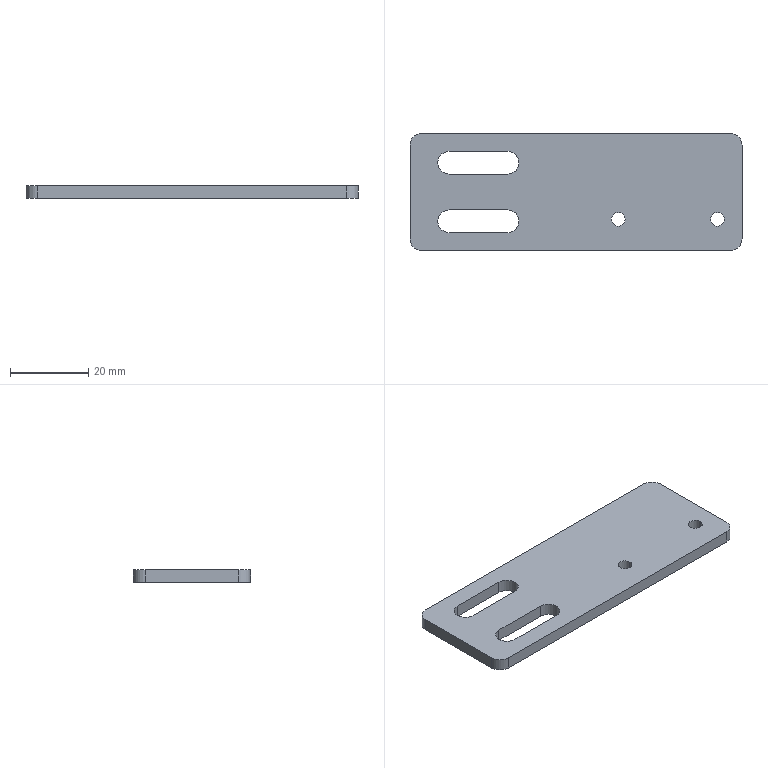Part | STEP file | J014-EBZ05-17-06 | 1 solid | 24 faces | box 85 x 30 x 3.2 mm | volume 7348 mm3 | cylinder 14 | plane 10 | commonest cylinder face diameters 5.8 x6 3.5 x4 6 x4
STEP:
#1=CARTESIAN_POINT('',(76.95,8.,0.));
#2=VERTEX_POINT('',#1);
#3=CARTESIAN_POINT('',(80.45,8.,0.));
#4=VERTEX_POINT('',#3);
#5=CARTESIAN_POINT('',(78.7,8.,0.));
#6=DIRECTION('',(0.,0.,1.));
#7=DIRECTION('',(1.,0.,0.));
#8=AXIS2_PLACEMENT_3D('',#5,#6,#7);
#9=CIRCLE('',#8,1.75);
#10=EDGE_CURVE('',#2,#4,#9,.T.);
#11=ORIENTED_EDGE('',*,*,#10,.F.);
#12=CARTESIAN_POINT('',(76.95,8.,3.2));
#13=VERTEX_POINT('',#12);
#14=CARTESIAN_POINT('',(76.95,8.,0.));
#15=DIRECTION('',(0.,0.,1.));
#16=VECTOR('',#15,1000.);
#17=LINE('',#14,#16);
#18=EDGE_CURVE('',#2,#13,#17,.T.);
#19=ORIENTED_EDGE('',*,*,#18,.T.);
#20=CARTESIAN_POINT('',(80.45,8.,3.2));
#21=VERTEX_POINT('',#20);
#22=CARTESIAN_POINT('',(78.7,8.,3.2));
#23=DIRECTION('',(0.,0.,-1.));
#24=DIRECTION('',(-1.,0.,0.));
#25=AXIS2_PLACEMENT_3D('',#22,#23,#24);
#26=CIRCLE('',#25,1.75);
#27=EDGE_CURVE('',#21,#13,#26,.T.);
#28=ORIENTED_EDGE('',*,*,#27,.F.);
#29=CARTESIAN_POINT('',(80.45,8.,0.));
#30=DIRECTION('',(0.,0.,1.));
#31=VECTOR('',#30,1000.);
#32=LINE('',#29,#31);
#33=EDGE_CURVE('',#4,#21,#32,.T.);
#34=ORIENTED_EDGE('',*,*,#33,.F.);
#35=EDGE_LOOP('',(#11,#19,#28,#34));
#36=FACE_OUTER_BOUND('',#35,.T.);
#37=CARTESIAN_POINT('',(78.7,8.,0.));
#38=DIRECTION('',(0.,0.,1.));
#39=DIRECTION('',(1.,0.,0.));
#40=AXIS2_PLACEMENT_3D('',#37,#38,#39);
#41=CYLINDRICAL_SURFACE('',#40,1.75);
#42=ADVANCED_FACE('',(#36),#41,.F.);
#43=CARTESIAN_POINT('',(51.55,8.,0.));
#44=VERTEX_POINT('',#43);
#45=CARTESIAN_POINT('',(55.05,8.,0.));
#46=VERTEX_POINT('',#45);
#47=CARTESIAN_POINT('',(53.3,8.,0.));
#48=DIRECTION('',(0.,0.,1.));
#49=DIRECTION('',(1.,0.,0.));
#50=AXIS2_PLACEMENT_3D('',#47,#48,#49);
#51=CIRCLE('',#50,1.75);
#52=EDGE_CURVE('',#44,#46,#51,.T.);
#53=ORIENTED_EDGE('',*,*,#52,.F.);
#54=CARTESIAN_POINT('',(51.55,8.,3.2));
#55=VERTEX_POINT('',#54);
#56=CARTESIAN_POINT('',(51.55,8.,0.));
#57=DIRECTION('',(0.,0.,1.));
#58=VECTOR('',#57,1000.);
#59=LINE('',#56,#58);
#60=EDGE_CURVE('',#44,#55,#59,.T.);
#61=ORIENTED_EDGE('',*,*,#60,.T.);
#62=CARTESIAN_POINT('',(55.05,8.,3.2));
#63=VERTEX_POINT('',#62);
#64=CARTESIAN_POINT('',(53.3,8.,3.2));
#65=DIRECTION('',(0.,0.,-1.));
#66=DIRECTION('',(-1.,0.,0.));
#67=AXIS2_PLACEMENT_3D('',#64,#65,#66);
#68=CIRCLE('',#67,1.75);
#69=EDGE_CURVE('',#63,#55,#68,.T.);
#70=ORIENTED_EDGE('',*,*,#69,.F.);
#71=CARTESIAN_POINT('',(55.05,8.,0.));
#72=DIRECTION('',(0.,0.,1.));
#73=VECTOR('',#72,1000.);
#74=LINE('',#71,#73);
#75=EDGE_CURVE('',#46,#63,#74,.T.);
#76=ORIENTED_EDGE('',*,*,#75,.F.);
#77=EDGE_LOOP('',(#53,#61,#70,#76));
#78=FACE_OUTER_BOUND('',#77,.T.);
#79=CARTESIAN_POINT('',(53.3,8.,0.));
#80=DIRECTION('',(0.,0.,1.));
#81=DIRECTION('',(1.,0.,0.));
#82=AXIS2_PLACEMENT_3D('',#79,#80,#81);
#83=CYLINDRICAL_SURFACE('',#82,1.75);
#84=ADVANCED_FACE('',(#78),#83,.F.);
#85=CARTESIAN_POINT('',(7.1,22.5,3.2));
#86=VERTEX_POINT('',#85);
#87=CARTESIAN_POINT('',(10.,25.4,3.2));
#88=VERTEX_POINT('',#87);
#89=CARTESIAN_POINT('',(10.,22.5,3.2));
#90=DIRECTION('',(0.,0.,-1.));
#91=DIRECTION('',(-1.,0.,0.));
#92=AXIS2_PLACEMENT_3D('',#89,#90,#91);
#93=CIRCLE('',#92,2.9);
#94=EDGE_CURVE('',#86,#88,#93,.T.);
#95=ORIENTED_EDGE('',*,*,#94,.F.);
#96=CARTESIAN_POINT('',(7.1,22.5,0.));
#97=VERTEX_POINT('',#96);
#98=CARTESIAN_POINT('',(7.1,22.5,3.2));
#99=DIRECTION('',(0.,0.,-1.));
#100=VECTOR('',#99,1000.);
#101=LINE('',#98,#100);
#102=EDGE_CURVE('',#86,#97,#101,.T.);
#103=ORIENTED_EDGE('',*,*,#102,.T.);
#104=CARTESIAN_POINT('',(10.,25.4,0.));
#105=VERTEX_POINT('',#104);
#106=CARTESIAN_POINT('',(10.,22.5,0.));
#107=DIRECTION('',(0.,0.,1.));
#108=DIRECTION('',(1.,0.,0.));
#109=AXIS2_PLACEMENT_3D('',#106,#107,#108);
#110=CIRCLE('',#109,2.9);
#111=EDGE_CURVE('',#105,#97,#110,.T.);
#112=ORIENTED_EDGE('',*,*,#111,.F.);
#113=CARTESIAN_POINT('',(10.,25.4,3.2));
#114=DIRECTION('',(0.,0.,-1.));
#115=VECTOR('',#114,1000.);
#116=LINE('',#113,#115);
#117=EDGE_CURVE('',#88,#105,#116,.T.);
#118=ORIENTED_EDGE('',*,*,#117,.F.);
#119=EDGE_LOOP('',(#95,#103,#112,#118));
#120=FACE_OUTER_BOUND('',#119,.T.);
#121=CARTESIAN_POINT('',(10.,22.5,3.2));
#122=DIRECTION('',(0.,0.,-1.));
#123=DIRECTION('',(-1.,0.,0.));
#124=AXIS2_PLACEMENT_3D('',#121,#122,#123);
#125=CYLINDRICAL_SURFACE('',#124,2.9);
#126=ADVANCED_FACE('',(#120),#125,.F.);
#127=CARTESIAN_POINT('',(7.1,7.5,3.2));
#128=VERTEX_POINT('',#127);
#129=CARTESIAN_POINT('',(10.,10.4,3.2));
#130=VERTEX_POINT('',#129);
#131=CARTESIAN_POINT('',(10.,7.5,3.2));
#132=DIRECTION('',(0.,0.,-1.));
#133=DIRECTION('',(-1.,0.,0.));
#134=AXIS2_PLACEMENT_3D('',#131,#132,#133);
#135=CIRCLE('',#134,2.9);
#136=EDGE_CURVE('',#128,#130,#135,.T.);
#137=ORIENTED_EDGE('',*,*,#136,.F.);
#138=CARTESIAN_POINT('',(7.1,7.5,0.));
#139=VERTEX_POINT('',#138);
#140=CARTESIAN_POINT('',(7.1,7.5,3.2));
#141=DIRECTION('',(0.,0.,-1.));
#142=VECTOR('',#141,1000.);
#143=LINE('',#140,#142);
#144=EDGE_CURVE('',#128,#139,#143,.T.);
#145=ORIENTED_EDGE('',*,*,#144,.T.);
#146=CARTESIAN_POINT('',(10.,10.4,0.));
#147=VERTEX_POINT('',#146);
#148=CARTESIAN_POINT('',(10.,7.5,0.));
#149=DIRECTION('',(0.,0.,1.));
#150=DIRECTION('',(1.,0.,0.));
#151=AXIS2_PLACEMENT_3D('',#148,#149,#150);
#152=CIRCLE('',#151,2.9);
#153=EDGE_CURVE('',#147,#139,#152,.T.);
#154=ORIENTED_EDGE('',*,*,#153,.F.);
#155=CARTESIAN_POINT('',(10.,10.4,3.2));
#156=DIRECTION('',(0.,0.,-1.));
#157=VECTOR('',#156,1000.);
#158=LINE('',#155,#157);
#159=EDGE_CURVE('',#130,#147,#158,.T.);
#160=ORIENTED_EDGE('',*,*,#159,.F.);
#161=EDGE_LOOP('',(#137,#145,#154,#160));
#162=FACE_OUTER_BOUND('',#161,.T.);
#163=CARTESIAN_POINT('',(10.,7.5,3.2));
#164=DIRECTION('',(0.,0.,-1.));
#165=DIRECTION('',(-1.,0.,0.));
#166=AXIS2_PLACEMENT_3D('',#163,#164,#165);
#167=CYLINDRICAL_SURFACE('',#166,2.9);
#168=ADVANCED_FACE('',(#162),#167,.F.);
#169=CARTESIAN_POINT('',(78.7,8.,0.));
#170=DIRECTION('',(0.,0.,1.));
#171=DIRECTION('',(1.,0.,0.));
#172=AXIS2_PLACEMENT_3D('',#169,#170,#171);
#173=CIRCLE('',#172,1.75);
#174=EDGE_CURVE('',#4,#2,#173,.T.);
#175=ORIENTED_EDGE('',*,*,#174,.T.);
#176=ORIENTED_EDGE('',*,*,#10,.T.);
#177=EDGE_LOOP('',(#175,#176));
#178=FACE_BOUND('',#177,.T.);
#179=CARTESIAN_POINT('',(53.3,8.,0.));
#180=DIRECTION('',(0.,0.,1.));
#181=DIRECTION('',(1.,0.,0.));
#182=AXIS2_PLACEMENT_3D('',#179,#180,#181);
#183=CIRCLE('',#182,1.75);
#184=EDGE_CURVE('',#46,#44,#183,.T.);
#185=ORIENTED_EDGE('',*,*,#184,.T.);
#186=ORIENTED_EDGE('',*,*,#52,.T.);
#187=EDGE_LOOP('',(#185,#186));
#188=FACE_BOUND('',#187,.T.);
#189=CARTESIAN_POINT('',(85.,3.,0.));
#190=VERTEX_POINT('',#189);
#191=CARTESIAN_POINT('',(85.,27.,0.));
#192=VERTEX_POINT('',#191);
#193=CARTESIAN_POINT('',(85.,15.,0.));
#194=DIRECTION('',(0.,1.,0.));
#195=VECTOR('',#194,1000.);
#196=LINE('',#193,#195);
#197=EDGE_CURVE('',#190,#192,#196,.T.);
#198=ORIENTED_EDGE('',*,*,#197,.F.);
#199=CARTESIAN_POINT('',(82.,0.,0.));
#200=VERTEX_POINT('',#199);
#201=CARTESIAN_POINT('',(82.,3.,0.));
#202=DIRECTION('',(0.,0.,-1.));
#203=DIRECTION('',(-1.,0.,0.));
#204=AXIS2_PLACEMENT_3D('',#201,#202,#203);
#205=CIRCLE('',#204,3.);
#206=EDGE_CURVE('',#190,#200,#205,.T.);
#207=ORIENTED_EDGE('',*,*,#206,.T.);
#208=CARTESIAN_POINT('',(3.,0.,0.));
#209=VERTEX_POINT('',#208);
#210=CARTESIAN_POINT('',(42.5,0.,0.));
#211=DIRECTION('',(1.,0.,0.));
#212=VECTOR('',#211,1000.);
#213=LINE('',#210,#212);
#214=EDGE_CURVE('',#209,#200,#213,.T.);
#215=ORIENTED_EDGE('',*,*,#214,.F.);
#216=CARTESIAN_POINT('',(0.,3.,0.));
#217=VERTEX_POINT('',#216);
#218=CARTESIAN_POINT('',(3.,3.,0.));
#219=DIRECTION('',(0.,0.,-1.));
#220=DIRECTION('',(-1.,0.,0.));
#221=AXIS2_PLACEMENT_3D('',#218,#219,#220);
#222=CIRCLE('',#221,3.);
#223=EDGE_CURVE('',#209,#217,#222,.T.);
#224=ORIENTED_EDGE('',*,*,#223,.T.);
#225=CARTESIAN_POINT('',(0.,27.,0.));
#226=VERTEX_POINT('',#225);
#227=CARTESIAN_POINT('',(0.,15.,0.));
#228=DIRECTION('',(0.,-1.,0.));
#229=VECTOR('',#228,1000.);
#230=LINE('',#227,#229);
#231=EDGE_CURVE('',#226,#217,#230,.T.);
#232=ORIENTED_EDGE('',*,*,#231,.F.);
#233=CARTESIAN_POINT('',(3.,30.,0.));
#234=VERTEX_POINT('',#233);
#235=CARTESIAN_POINT('',(3.,27.,0.));
#236=DIRECTION('',(0.,0.,-1.));
#237=DIRECTION('',(-1.,0.,0.));
#238=AXIS2_PLACEMENT_3D('',#235,#236,#237);
#239=CIRCLE('',#238,3.);
#240=EDGE_CURVE('',#226,#234,#239,.T.);
#241=ORIENTED_EDGE('',*,*,#240,.T.);
#242=CARTESIAN_POINT('',(82.,30.,0.));
#243=VERTEX_POINT('',#242);
#244=CARTESIAN_POINT('',(42.5,30.,0.));
#245=DIRECTION('',(-1.,0.,0.));
#246=VECTOR('',#245,1000.);
#247=LINE('',#244,#246);
#248=EDGE_CURVE('',#243,#234,#247,.T.);
#249=ORIENTED_EDGE('',*,*,#248,.F.);
#250=CARTESIAN_POINT('',(82.,27.,0.));
#251=DIRECTION('',(0.,0.,-1.));
#252=DIRECTION('',(-1.,0.,0.));
#253=AXIS2_PLACEMENT_3D('',#250,#251,#252);
#254=CIRCLE('',#253,3.);
#255=EDGE_CURVE('',#243,#192,#254,.T.);
#256=ORIENTED_EDGE('',*,*,#255,.T.);
#257=EDGE_LOOP('',(#198,#207,#215,#224,#232,#241,#249,#256));
#258=FACE_OUTER_BOUND('',#257,.T.);
#259=CARTESIAN_POINT('',(10.,4.6,0.));
#260=VERTEX_POINT('',#259);
#261=CARTESIAN_POINT('',(25.,4.6,0.));
#262=VERTEX_POINT('',#261);
#263=CARTESIAN_POINT('',(17.5,4.6,0.));
#264=DIRECTION('',(1.,0.,0.));
#265=VECTOR('',#264,1000.);
#266=LINE('',#263,#265);
#267=EDGE_CURVE('',#260,#262,#266,.T.);
#268=ORIENTED_EDGE('',*,*,#267,.T.);
#269=CARTESIAN_POINT('',(25.,10.4,0.));
#270=VERTEX_POINT('',#269);
#271=CARTESIAN_POINT('',(25.,7.5,0.));
#272=DIRECTION('',(0.,0.,1.));
#273=DIRECTION('',(1.,0.,0.));
#274=AXIS2_PLACEMENT_3D('',#271,#272,#273);
#275=CIRCLE('',#274,2.9);
#276=EDGE_CURVE('',#262,#270,#275,.T.);
#277=ORIENTED_EDGE('',*,*,#276,.T.);
#278=CARTESIAN_POINT('',(17.5,10.4,0.));
#279=DIRECTION('',(-1.,0.,0.));
#280=VECTOR('',#279,1000.);
#281=LINE('',#278,#280);
#282=EDGE_CURVE('',#270,#147,#281,.T.);
#283=ORIENTED_EDGE('',*,*,#282,.T.);
#284=ORIENTED_EDGE('',*,*,#153,.T.);
#285=CARTESIAN_POINT('',(10.,7.5,0.));
#286=DIRECTION('',(0.,0.,1.));
#287=DIRECTION('',(1.,0.,0.));
#288=AXIS2_PLACEMENT_3D('',#285,#286,#287);
#289=CIRCLE('',#288,2.9);
#290=EDGE_CURVE('',#139,#260,#289,.T.);
#291=ORIENTED_EDGE('',*,*,#290,.T.);
#292=EDGE_LOOP('',(#268,#277,#283,#284,#291));
#293=FACE_BOUND('',#292,.T.);
#294=CARTESIAN_POINT('',(10.,19.6,0.));
#295=VERTEX_POINT('',#294);
#296=CARTESIAN_POINT('',(25.,19.6,0.));
#297=VERTEX_POINT('',#296);
#298=CARTESIAN_POINT('',(17.5,19.6,0.));
#299=DIRECTION('',(1.,0.,0.));
#300=VECTOR('',#299,1000.);
#301=LINE('',#298,#300);
#302=EDGE_CURVE('',#295,#297,#301,.T.);
#303=ORIENTED_EDGE('',*,*,#302,.T.);
#304=CARTESIAN_POINT('',(25.,25.4,0.));
#305=VERTEX_POINT('',#304);
#306=CARTESIAN_POINT('',(25.,22.5,0.));
#307=DIRECTION('',(0.,0.,1.));
#308=DIRECTION('',(1.,0.,0.));
#309=AXIS2_PLACEMENT_3D('',#306,#307,#308);
#310=CIRCLE('',#309,2.9);
#311=EDGE_CURVE('',#297,#305,#310,.T.);
#312=ORIENTED_EDGE('',*,*,#311,.T.);
#313=CARTESIAN_POINT('',(17.5,25.4,0.));
#314=DIRECTION('',(-1.,0.,0.));
#315=VECTOR('',#314,1000.);
#316=LINE('',#313,#315);
#317=EDGE_CURVE('',#305,#105,#316,.T.);
#318=ORIENTED_EDGE('',*,*,#317,.T.);
#319=ORIENTED_EDGE('',*,*,#111,.T.);
#320=CARTESIAN_POINT('',(10.,22.5,0.));
#321=DIRECTION('',(0.,0.,1.));
#322=DIRECTION('',(1.,0.,0.));
#323=AXIS2_PLACEMENT_3D('',#320,#321,#322);
#324=CIRCLE('',#323,2.9);
#325=EDGE_CURVE('',#97,#295,#324,.T.);
#326=ORIENTED_EDGE('',*,*,#325,.T.);
#327=EDGE_LOOP('',(#303,#312,#318,#319,#326));
#328=FACE_BOUND('',#327,.T.);
#329=CARTESIAN_POINT('',(42.5,15.,0.));
#330=DIRECTION('',(0.,0.,-1.));
#331=DIRECTION('',(-1.,0.,0.));
#332=AXIS2_PLACEMENT_3D('',#329,#330,#331);
#333=PLANE('',#332);
#334=ADVANCED_FACE('',(#178,#188,#258,#293,#328),#333,.T.);
#335=ORIENTED_EDGE('',*,*,#27,.T.);
#336=CARTESIAN_POINT('',(78.7,8.,3.2));
#337=DIRECTION('',(0.,0.,-1.));
#338=DIRECTION('',(-1.,0.,0.));
#339=AXIS2_PLACEMENT_3D('',#336,#337,#338);
#340=CIRCLE('',#339,1.75);
#341=EDGE_CURVE('',#13,#21,#340,.T.);
#342=ORIENTED_EDGE('',*,*,#341,.T.);
#343=EDGE_LOOP('',(#335,#342));
#344=FACE_BOUND('',#343,.T.);
#345=ORIENTED_EDGE('',*,*,#69,.T.);
#346=CARTESIAN_POINT('',(53.3,8.,3.2));
#347=DIRECTION('',(0.,0.,-1.));
#348=DIRECTION('',(-1.,0.,0.));
#349=AXIS2_PLACEMENT_3D('',#346,#347,#348);
#350=CIRCLE('',#349,1.75);
#351=EDGE_CURVE('',#55,#63,#350,.T.);
#352=ORIENTED_EDGE('',*,*,#351,.T.);
#353=EDGE_LOOP('',(#345,#352));
#354=FACE_BOUND('',#353,.T.);
#355=CARTESIAN_POINT('',(82.,0.,3.2));
#356=VERTEX_POINT('',#355);
#357=CARTESIAN_POINT('',(3.,0.,3.2));
#358=VERTEX_POINT('',#357);
#359=CARTESIAN_POINT('',(42.5,0.,3.2));
#360=DIRECTION('',(-1.,0.,0.));
#361=VECTOR('',#360,1000.);
#362=LINE('',#359,#361);
#363=EDGE_CURVE('',#356,#358,#362,.T.);
#364=ORIENTED_EDGE('',*,*,#363,.F.);
#365=CARTESIAN_POINT('',(85.,3.,3.2));
#366=VERTEX_POINT('',#365);
#367=CARTESIAN_POINT('',(82.,3.,3.2));
#368=DIRECTION('',(0.,0.,1.));
#369=DIRECTION('',(1.,0.,0.));
#370=AXIS2_PLACEMENT_3D('',#367,#368,#369);
#371=CIRCLE('',#370,3.);
#372=EDGE_CURVE('',#356,#366,#371,.T.);
#373=ORIENTED_EDGE('',*,*,#372,.T.);
#374=CARTESIAN_POINT('',(85.,27.,3.2));
#375=VERTEX_POINT('',#374);
#376=CARTESIAN_POINT('',(85.,15.,3.2));
#377=DIRECTION('',(0.,-1.,0.));
#378=VECTOR('',#377,1000.);
#379=LINE('',#376,#378);
#380=EDGE_CURVE('',#375,#366,#379,.T.);
#381=ORIENTED_EDGE('',*,*,#380,.F.);
#382=CARTESIAN_POINT('',(82.,30.,3.2));
#383=VERTEX_POINT('',#382);
#384=CARTESIAN_POINT('',(82.,27.,3.2));
#385=DIRECTION('',(0.,0.,1.));
#386=DIRECTION('',(1.,0.,0.));
#387=AXIS2_PLACEMENT_3D('',#384,#385,#386);
#388=CIRCLE('',#387,3.);
#389=EDGE_CURVE('',#375,#383,#388,.T.);
#390=ORIENTED_EDGE('',*,*,#389,.T.);
#391=CARTESIAN_POINT('',(3.,30.,3.2));
#392=VERTEX_POINT('',#391);
#393=CARTESIAN_POINT('',(42.5,30.,3.2));
#394=DIRECTION('',(1.,0.,0.));
#395=VECTOR('',#394,1000.);
#396=LINE('',#393,#395);
#397=EDGE_CURVE('',#392,#383,#396,.T.);
#398=ORIENTED_EDGE('',*,*,#397,.F.);
#399=CARTESIAN_POINT('',(0.,27.,3.2));
#400=VERTEX_POINT('',#399);
#401=CARTESIAN_POINT('',(3.,27.,3.2));
#402=DIRECTION('',(0.,0.,1.));
#403=DIRECTION('',(1.,0.,0.));
#404=AXIS2_PLACEMENT_3D('',#401,#402,#403);
#405=CIRCLE('',#404,3.);
#406=EDGE_CURVE('',#392,#400,#405,.T.);
#407=ORIENTED_EDGE('',*,*,#406,.T.);
#408=CARTESIAN_POINT('',(0.,3.,3.2));
#409=VERTEX_POINT('',#408);
#410=CARTESIAN_POINT('',(0.,15.,3.2));
#411=DIRECTION('',(0.,1.,0.));
#412=VECTOR('',#411,1000.);
#413=LINE('',#410,#412);
#414=EDGE_CURVE('',#409,#400,#413,.T.);
#415=ORIENTED_EDGE('',*,*,#414,.F.);
#416=CARTESIAN_POINT('',(3.,3.,3.2));
#417=DIRECTION('',(0.,0.,1.));
#418=DIRECTION('',(1.,0.,0.));
#419=AXIS2_PLACEMENT_3D('',#416,#417,#418);
#420=CIRCLE('',#419,3.);
#421=EDGE_CURVE('',#409,#358,#420,.T.);
#422=ORIENTED_EDGE('',*,*,#421,.T.);
#423=EDGE_LOOP('',(#364,#373,#381,#390,#398,#407,#415,#422));
#424=FACE_OUTER_BOUND('',#423,.T.);
#425=CARTESIAN_POINT('',(25.,10.4,3.2));
#426=VERTEX_POINT('',#425);
#427=CARTESIAN_POINT('',(17.5,10.4,3.2));
#428=DIRECTION('',(1.,0.,0.));
#429=VECTOR('',#428,1000.);
#430=LINE('',#427,#429);
#431=EDGE_CURVE('',#130,#426,#430,.T.);
#432=ORIENTED_EDGE('',*,*,#431,.T.);
#433=CARTESIAN_POINT('',(25.,4.6,3.2));
#434=VERTEX_POINT('',#433);
#435=CARTESIAN_POINT('',(25.,7.5,3.2));
#436=DIRECTION('',(0.,0.,-1.));
#437=DIRECTION('',(-1.,0.,0.));
#438=AXIS2_PLACEMENT_3D('',#435,#436,#437);
#439=CIRCLE('',#438,2.9);
#440=EDGE_CURVE('',#426,#434,#439,.T.);
#441=ORIENTED_EDGE('',*,*,#440,.T.);
#442=CARTESIAN_POINT('',(10.,4.6,3.2));
#443=VERTEX_POINT('',#442);
#444=CARTESIAN_POINT('',(17.5,4.6,3.2));
#445=DIRECTION('',(-1.,0.,0.));
#446=VECTOR('',#445,1000.);
#447=LINE('',#444,#446);
#448=EDGE_CURVE('',#434,#443,#447,.T.);
#449=ORIENTED_EDGE('',*,*,#448,.T.);
#450=CARTESIAN_POINT('',(10.,7.5,3.2));
#451=DIRECTION('',(0.,0.,-1.));
#452=DIRECTION('',(-1.,0.,0.));
#453=AXIS2_PLACEMENT_3D('',#450,#451,#452);
#454=CIRCLE('',#453,2.9);
#455=EDGE_CURVE('',#443,#128,#454,.T.);
#456=ORIENTED_EDGE('',*,*,#455,.T.);
#457=ORIENTED_EDGE('',*,*,#136,.T.);
#458=EDGE_LOOP('',(#432,#441,#449,#456,#457));
#459=FACE_BOUND('',#458,.T.);
#460=CARTESIAN_POINT('',(25.,25.4,3.2));
#461=VERTEX_POINT('',#460);
#462=CARTESIAN_POINT('',(17.5,25.4,3.2));
#463=DIRECTION('',(1.,0.,0.));
#464=VECTOR('',#463,1000.);
#465=LINE('',#462,#464);
#466=EDGE_CURVE('',#88,#461,#465,.T.);
#467=ORIENTED_EDGE('',*,*,#466,.T.);
#468=CARTESIAN_POINT('',(25.,19.6,3.2));
#469=VERTEX_POINT('',#468);
#470=CARTESIAN_POINT('',(25.,22.5,3.2));
#471=DIRECTION('',(0.,0.,-1.));
#472=DIRECTION('',(-1.,0.,0.));
#473=AXIS2_PLACEMENT_3D('',#470,#471,#472);
#474=CIRCLE('',#473,2.9);
#475=EDGE_CURVE('',#461,#469,#474,.T.);
#476=ORIENTED_EDGE('',*,*,#475,.T.);
#477=CARTESIAN_POINT('',(10.,19.6,3.2));
#478=VERTEX_POINT('',#477);
#479=CARTESIAN_POINT('',(17.5,19.6,3.2));
#480=DIRECTION('',(-1.,0.,0.));
#481=VECTOR('',#480,1000.);
#482=LINE('',#479,#481);
#483=EDGE_CURVE('',#469,#478,#482,.T.);
#484=ORIENTED_EDGE('',*,*,#483,.T.);
#485=CARTESIAN_POINT('',(10.,22.5,3.2));
#486=DIRECTION('',(0.,0.,-1.));
#487=DIRECTION('',(-1.,0.,0.));
#488=AXIS2_PLACEMENT_3D('',#485,#486,#487);
#489=CIRCLE('',#488,2.9);
#490=EDGE_CURVE('',#478,#86,#489,.T.);
#491=ORIENTED_EDGE('',*,*,#490,.T.);
#492=ORIENTED_EDGE('',*,*,#94,.T.);
#493=EDGE_LOOP('',(#467,#476,#484,#491,#492));
#494=FACE_BOUND('',#493,.T.);
#495=CARTESIAN_POINT('',(42.5,15.,3.2));
#496=DIRECTION('',(0.,0.,1.));
#497=DIRECTION('',(1.,0.,0.));
#498=AXIS2_PLACEMENT_3D('',#495,#496,#497);
#499=PLANE('',#498);
#500=ADVANCED_FACE('',(#344,#354,#424,#459,#494),#499,.T.);
#501=ORIENTED_EDGE('',*,*,#214,.T.);
#502=CARTESIAN_POINT('',(82.,0.,3.2));
#503=DIRECTION('',(0.,0.,1.));
#504=VECTOR('',#503,1000.);
#505=LINE('',#502,#504);
#506=EDGE_CURVE('',#200,#356,#505,.T.);
#507=ORIENTED_EDGE('',*,*,#506,.T.);
#508=ORIENTED_EDGE('',*,*,#363,.T.);
#509=CARTESIAN_POINT('',(3.,0.,3.2));
#510=DIRECTION('',(0.,0.,-1.));
#511=VECTOR('',#510,1000.);
#512=LINE('',#509,#511);
#513=EDGE_CURVE('',#358,#209,#512,.T.);
#514=ORIENTED_EDGE('',*,*,#513,.T.);
#515=EDGE_LOOP('',(#501,#507,#508,#514));
#516=FACE_OUTER_BOUND('',#515,.T.);
#517=CARTESIAN_POINT('',(42.5,0.,3.2));
#518=DIRECTION('',(0.,-1.,0.));
#519=DIRECTION('',(0.,0.,1.));
#520=AXIS2_PLACEMENT_3D('',#517,#518,#519);
#521=PLANE('',#520);
#522=ADVANCED_FACE('',(#516),#521,.T.);
#523=ORIENTED_EDGE('',*,*,#380,.T.);
#524=CARTESIAN_POINT('',(85.,3.,3.2));
#525=DIRECTION('',(0.,0.,-1.));
#526=VECTOR('',#525,1000.);
#527=LINE('',#524,#526);
#528=EDGE_CURVE('',#366,#190,#527,.T.);
#529=ORIENTED_EDGE('',*,*,#528,.T.);
#530=ORIENTED_EDGE('',*,*,#197,.T.);
#531=CARTESIAN_POINT('',(85.,27.,3.2));
#532=DIRECTION('',(0.,0.,1.));
#533=VECTOR('',#532,1000.);
#534=LINE('',#531,#533);
#535=EDGE_CURVE('',#192,#375,#534,.T.);
#536=ORIENTED_EDGE('',*,*,#535,.T.);
#537=EDGE_LOOP('',(#523,#529,#530,#536));
#538=FACE_OUTER_BOUND('',#537,.T.);
#539=CARTESIAN_POINT('',(85.,15.,3.2));
#540=DIRECTION('',(1.,0.,0.));
#541=DIRECTION('',(0.,0.,-1.));
#542=AXIS2_PLACEMENT_3D('',#539,#540,#541);
#543=PLANE('',#542);
#544=ADVANCED_FACE('',(#538),#543,.T.);
#545=ORIENTED_EDGE('',*,*,#397,.T.);
#546=CARTESIAN_POINT('',(82.,30.,3.2));
#547=DIRECTION('',(0.,0.,-1.));
#548=VECTOR('',#547,1000.);
#549=LINE('',#546,#548);
#550=EDGE_CURVE('',#383,#243,#549,.T.);
#551=ORIENTED_EDGE('',*,*,#550,.T.);
#552=ORIENTED_EDGE('',*,*,#248,.T.);
#553=CARTESIAN_POINT('',(3.,30.,3.2));
#554=DIRECTION('',(0.,0.,1.));
#555=VECTOR('',#554,1000.);
#556=LINE('',#553,#555);
#557=EDGE_CURVE('',#234,#392,#556,.T.);
#558=ORIENTED_EDGE('',*,*,#557,.T.);
#559=EDGE_LOOP('',(#545,#551,#552,#558));
#560=FACE_OUTER_BOUND('',#559,.T.);
#561=CARTESIAN_POINT('',(42.5,30.,3.2));
#562=DIRECTION('',(0.,1.,0.));
#563=DIRECTION('',(0.,0.,-1.));
#564=AXIS2_PLACEMENT_3D('',#561,#562,#563);
#565=PLANE('',#564);
#566=ADVANCED_FACE('',(#560),#565,.T.);
#567=ORIENTED_EDGE('',*,*,#231,.T.);
#568=CARTESIAN_POINT('',(0.,3.,3.2));
#569=DIRECTION('',(0.,0.,1.));
#570=VECTOR('',#569,1000.);
#571=LINE('',#568,#570);
#572=EDGE_CURVE('',#217,#409,#571,.T.);
#573=ORIENTED_EDGE('',*,*,#572,.T.);
#574=ORIENTED_EDGE('',*,*,#414,.T.);
#575=CARTESIAN_POINT('',(0.,27.,3.2));
#576=DIRECTION('',(0.,0.,-1.));
#577=VECTOR('',#576,1000.);
#578=LINE('',#575,#577);
#579=EDGE_CURVE('',#400,#226,#578,.T.);
#580=ORIENTED_EDGE('',*,*,#579,.T.);
#581=EDGE_LOOP('',(#567,#573,#574,#580));
#582=FACE_OUTER_BOUND('',#581,.T.);
#583=CARTESIAN_POINT('',(0.,15.,3.2));
#584=DIRECTION('',(-1.,0.,0.));
#585=DIRECTION('',(0.,0.,1.));
#586=AXIS2_PLACEMENT_3D('',#583,#584,#585);
#587=PLANE('',#586);
#588=ADVANCED_FACE('',(#582),#587,.T.);
#589=CARTESIAN_POINT('',(10.,4.6,3.2));
#590=DIRECTION('',(0.,0.,-1.));
#591=VECTOR('',#590,1000.);
#592=LINE('',#589,#591);
#593=EDGE_CURVE('',#443,#260,#592,.T.);
#594=ORIENTED_EDGE('',*,*,#593,.F.);
#595=ORIENTED_EDGE('',*,*,#448,.F.);
#596=CARTESIAN_POINT('',(25.,4.6,3.2));
#597=DIRECTION('',(0.,0.,-1.));
#598=VECTOR('',#597,1000.);
#599=LINE('',#596,#598);
#600=EDGE_CURVE('',#434,#262,#599,.T.);
#601=ORIENTED_EDGE('',*,*,#600,.T.);
#602=ORIENTED_EDGE('',*,*,#267,.F.);
#603=EDGE_LOOP('',(#594,#595,#601,#602));
#604=FACE_OUTER_BOUND('',#603,.T.);
#605=CARTESIAN_POINT('',(17.5,4.6,3.2));
#606=DIRECTION('',(0.,-1.,0.));
#607=DIRECTION('',(0.,0.,1.));
#608=AXIS2_PLACEMENT_3D('',#605,#606,#607);
#609=PLANE('',#608);
#610=ADVANCED_FACE('',(#604),#609,.F.);
#611=CARTESIAN_POINT('',(25.,10.4,3.2));
#612=DIRECTION('',(0.,0.,-1.));
#613=VECTOR('',#612,1000.);
#614=LINE('',#611,#613);
#615=EDGE_CURVE('',#426,#270,#614,.T.);
#616=ORIENTED_EDGE('',*,*,#615,.F.);
#617=ORIENTED_EDGE('',*,*,#431,.F.);
#618=ORIENTED_EDGE('',*,*,#159,.T.);
#619=ORIENTED_EDGE('',*,*,#282,.F.);
#620=EDGE_LOOP('',(#616,#617,#618,#619));
#621=FACE_OUTER_BOUND('',#620,.T.);
#622=CARTESIAN_POINT('',(17.5,10.4,3.2));
#623=DIRECTION('',(0.,1.,0.));
#624=DIRECTION('',(0.,0.,-1.));
#625=AXIS2_PLACEMENT_3D('',#622,#623,#624);
#626=PLANE('',#625);
#627=ADVANCED_FACE('',(#621),#626,.F.);
#628=ORIENTED_EDGE('',*,*,#440,.F.);
#629=ORIENTED_EDGE('',*,*,#615,.T.);
#630=ORIENTED_EDGE('',*,*,#276,.F.);
#631=ORIENTED_EDGE('',*,*,#600,.F.);
#632=EDGE_LOOP('',(#628,#629,#630,#631));
#633=FACE_OUTER_BOUND('',#632,.T.);
#634=CARTESIAN_POINT('',(25.,7.5,3.2));
#635=DIRECTION('',(0.,0.,-1.));
#636=DIRECTION('',(-1.,0.,0.));
#637=AXIS2_PLACEMENT_3D('',#634,#635,#636);
#638=CYLINDRICAL_SURFACE('',#637,2.9);
#639=ADVANCED_FACE('',(#633),#638,.F.);
#640=ORIENTED_EDGE('',*,*,#144,.F.);
#641=ORIENTED_EDGE('',*,*,#455,.F.);
#642=ORIENTED_EDGE('',*,*,#593,.T.);
#643=ORIENTED_EDGE('',*,*,#290,.F.);
#644=EDGE_LOOP('',(#640,#641,#642,#643));
#645=FACE_OUTER_BOUND('',#644,.T.);
#646=CARTESIAN_POINT('',(10.,7.5,3.2));
#647=DIRECTION('',(0.,0.,-1.));
#648=DIRECTION('',(-1.,0.,0.));
#649=AXIS2_PLACEMENT_3D('',#646,#647,#648);
#650=CYLINDRICAL_SURFACE('',#649,2.9);
#651=ADVANCED_FACE('',(#645),#650,.F.);
#652=CARTESIAN_POINT('',(10.,19.6,3.2));
#653=DIRECTION('',(0.,0.,-1.));
#654=VECTOR('',#653,1000.);
#655=LINE('',#652,#654);
#656=EDGE_CURVE('',#478,#295,#655,.T.);
#657=ORIENTED_EDGE('',*,*,#656,.F.);
#658=ORIENTED_EDGE('',*,*,#483,.F.);
#659=CARTESIAN_POINT('',(25.,19.6,3.2));
#660=DIRECTION('',(0.,0.,-1.));
#661=VECTOR('',#660,1000.);
#662=LINE('',#659,#661);
#663=EDGE_CURVE('',#469,#297,#662,.T.);
#664=ORIENTED_EDGE('',*,*,#663,.T.);
#665=ORIENTED_EDGE('',*,*,#302,.F.);
#666=EDGE_LOOP('',(#657,#658,#664,#665));
#667=FACE_OUTER_BOUND('',#666,.T.);
#668=CARTESIAN_POINT('',(17.5,19.6,3.2));
#669=DIRECTION('',(0.,-1.,0.));
#670=DIRECTION('',(0.,0.,1.));
#671=AXIS2_PLACEMENT_3D('',#668,#669,#670);
#672=PLANE('',#671);
#673=ADVANCED_FACE('',(#667),#672,.F.);
#674=CARTESIAN_POINT('',(25.,25.4,3.2));
#675=DIRECTION('',(0.,0.,-1.));
#676=VECTOR('',#675,1000.);
#677=LINE('',#674,#676);
#678=EDGE_CURVE('',#461,#305,#677,.T.);
#679=ORIENTED_EDGE('',*,*,#678,.F.);
#680=ORIENTED_EDGE('',*,*,#466,.F.);
#681=ORIENTED_EDGE('',*,*,#117,.T.);
#682=ORIENTED_EDGE('',*,*,#317,.F.);
#683=EDGE_LOOP('',(#679,#680,#681,#682));
#684=FACE_OUTER_BOUND('',#683,.T.);
#685=CARTESIAN_POINT('',(17.5,25.4,3.2));
#686=DIRECTION('',(0.,1.,0.));
#687=DIRECTION('',(0.,0.,-1.));
#688=AXIS2_PLACEMENT_3D('',#685,#686,#687);
#689=PLANE('',#688);
#690=ADVANCED_FACE('',(#684),#689,.F.);
#691=ORIENTED_EDGE('',*,*,#475,.F.);
#692=ORIENTED_EDGE('',*,*,#678,.T.);
#693=ORIENTED_EDGE('',*,*,#311,.F.);
#694=ORIENTED_EDGE('',*,*,#663,.F.);
#695=EDGE_LOOP('',(#691,#692,#693,#694));
#696=FACE_OUTER_BOUND('',#695,.T.);
#697=CARTESIAN_POINT('',(25.,22.5,3.2));
#698=DIRECTION('',(0.,0.,-1.));
#699=DIRECTION('',(-1.,0.,0.));
#700=AXIS2_PLACEMENT_3D('',#697,#698,#699);
#701=CYLINDRICAL_SURFACE('',#700,2.9);
#702=ADVANCED_FACE('',(#696),#701,.F.);
#703=ORIENTED_EDGE('',*,*,#102,.F.);
#704=ORIENTED_EDGE('',*,*,#490,.F.);
#705=ORIENTED_EDGE('',*,*,#656,.T.);
#706=ORIENTED_EDGE('',*,*,#325,.F.);
#707=EDGE_LOOP('',(#703,#704,#705,#706));
#708=FACE_OUTER_BOUND('',#707,.T.);
#709=CARTESIAN_POINT('',(10.,22.5,3.2));
#710=DIRECTION('',(0.,0.,-1.));
#711=DIRECTION('',(-1.,0.,0.));
#712=AXIS2_PLACEMENT_3D('',#709,#710,#711);
#713=CYLINDRICAL_SURFACE('',#712,2.9);
#714=ADVANCED_FACE('',(#708),#713,.F.);
#715=ORIENTED_EDGE('',*,*,#60,.F.);
#716=ORIENTED_EDGE('',*,*,#184,.F.);
#717=ORIENTED_EDGE('',*,*,#75,.T.);
#718=ORIENTED_EDGE('',*,*,#351,.F.);
#719=EDGE_LOOP('',(#715,#716,#717,#718));
#720=FACE_OUTER_BOUND('',#719,.T.);
#721=CARTESIAN_POINT('',(53.3,8.,0.));
#722=DIRECTION('',(0.,0.,1.));
#723=DIRECTION('',(1.,0.,0.));
#724=AXIS2_PLACEMENT_3D('',#721,#722,#723);
#725=CYLINDRICAL_SURFACE('',#724,1.75);
#726=ADVANCED_FACE('',(#720),#725,.F.);
#727=ORIENTED_EDGE('',*,*,#18,.F.);
#728=ORIENTED_EDGE('',*,*,#174,.F.);
#729=ORIENTED_EDGE('',*,*,#33,.T.);
#730=ORIENTED_EDGE('',*,*,#341,.F.);
#731=EDGE_LOOP('',(#727,#728,#729,#730));
#732=FACE_OUTER_BOUND('',#731,.T.);
#733=CARTESIAN_POINT('',(78.7,8.,0.));
#734=DIRECTION('',(0.,0.,1.));
#735=DIRECTION('',(1.,0.,0.));
#736=AXIS2_PLACEMENT_3D('',#733,#734,#735);
#737=CYLINDRICAL_SURFACE('',#736,1.75);
#738=ADVANCED_FACE('',(#732),#737,.F.);
#739=ORIENTED_EDGE('',*,*,#406,.F.);
#740=ORIENTED_EDGE('',*,*,#557,.F.);
#741=ORIENTED_EDGE('',*,*,#240,.F.);
#742=ORIENTED_EDGE('',*,*,#579,.F.);
#743=EDGE_LOOP('',(#739,#740,#741,#742));
#744=FACE_OUTER_BOUND('',#743,.T.);
#745=CARTESIAN_POINT('',(3.,27.,3.2));
#746=DIRECTION('',(0.,0.,-1.));
#747=DIRECTION('',(-1.,0.,0.));
#748=AXIS2_PLACEMENT_3D('',#745,#746,#747);
#749=CYLINDRICAL_SURFACE('',#748,3.);
#750=ADVANCED_FACE('',(#744),#749,.T.);
#751=ORIENTED_EDGE('',*,*,#421,.F.);
#752=ORIENTED_EDGE('',*,*,#572,.F.);
#753=ORIENTED_EDGE('',*,*,#223,.F.);
#754=ORIENTED_EDGE('',*,*,#513,.F.);
#755=EDGE_LOOP('',(#751,#752,#753,#754));
#756=FACE_OUTER_BOUND('',#755,.T.);
#757=CARTESIAN_POINT('',(3.,3.,3.2));
#758=DIRECTION('',(0.,0.,-1.));
#759=DIRECTION('',(-1.,0.,0.));
#760=AXIS2_PLACEMENT_3D('',#757,#758,#759);
#761=CYLINDRICAL_SURFACE('',#760,3.);
#762=ADVANCED_FACE('',(#756),#761,.T.);
#763=ORIENTED_EDGE('',*,*,#389,.F.);
#764=ORIENTED_EDGE('',*,*,#535,.F.);
#765=ORIENTED_EDGE('',*,*,#255,.F.);
#766=ORIENTED_EDGE('',*,*,#550,.F.);
#767=EDGE_LOOP('',(#763,#764,#765,#766));
#768=FACE_OUTER_BOUND('',#767,.T.);
#769=CARTESIAN_POINT('',(82.,27.,3.2));
#770=DIRECTION('',(0.,0.,-1.));
#771=DIRECTION('',(-1.,0.,0.));
#772=AXIS2_PLACEMENT_3D('',#769,#770,#771);
#773=CYLINDRICAL_SURFACE('',#772,3.);
#774=ADVANCED_FACE('',(#768),#773,.T.);
#775=ORIENTED_EDGE('',*,*,#372,.F.);
#776=ORIENTED_EDGE('',*,*,#506,.F.);
#777=ORIENTED_EDGE('',*,*,#206,.F.);
#778=ORIENTED_EDGE('',*,*,#528,.F.);
#779=EDGE_LOOP('',(#775,#776,#777,#778));
#780=FACE_OUTER_BOUND('',#779,.T.);
#781=CARTESIAN_POINT('',(82.,3.,3.2));
#782=DIRECTION('',(0.,0.,-1.));
#783=DIRECTION('',(-1.,0.,0.));
#784=AXIS2_PLACEMENT_3D('',#781,#782,#783);
#785=CYLINDRICAL_SURFACE('',#784,3.);
#786=ADVANCED_FACE('',(#780),#785,.T.);
#787=CLOSED_SHELL('',(#42,#84,#126,#168,#334,#500,#522,#544,#566,#588,#610,#627,#639,#651,#673,#690,#702,#714,#726,#738,#750,#762,#774,#786));
#788=MANIFOLD_SOLID_BREP('',#787);
#789=CARTESIAN_POINT('',(0.,0.,0.));
#790=DIRECTION('',(0.,0.,1.));
#791=DIRECTION('',(1.,0.,0.));
#792=AXIS2_PLACEMENT_3D('',#789,#790,#791);
#793=(LENGTH_UNIT()NAMED_UNIT(*)SI_UNIT(.MILLI.,.METRE.));
#794=UNCERTAINTY_MEASURE_WITH_UNIT(LENGTH_MEASURE(0.00001),#793,'','');
#795=(NAMED_UNIT(*)PLANE_ANGLE_UNIT()SI_UNIT($,.RADIAN.));
#796=(NAMED_UNIT(*)SI_UNIT($,.STERADIAN.)SOLID_ANGLE_UNIT());
#797=(GEOMETRIC_REPRESENTATION_CONTEXT(3)GLOBAL_UNCERTAINTY_ASSIGNED_CONTEXT((#794))GLOBAL_UNIT_ASSIGNED_CONTEXT((#793,#795,#796))REPRESENTATION_CONTEXT('',''));
#798=ADVANCED_BREP_SHAPE_REPRESENTATION('',(#788,#792),#797);